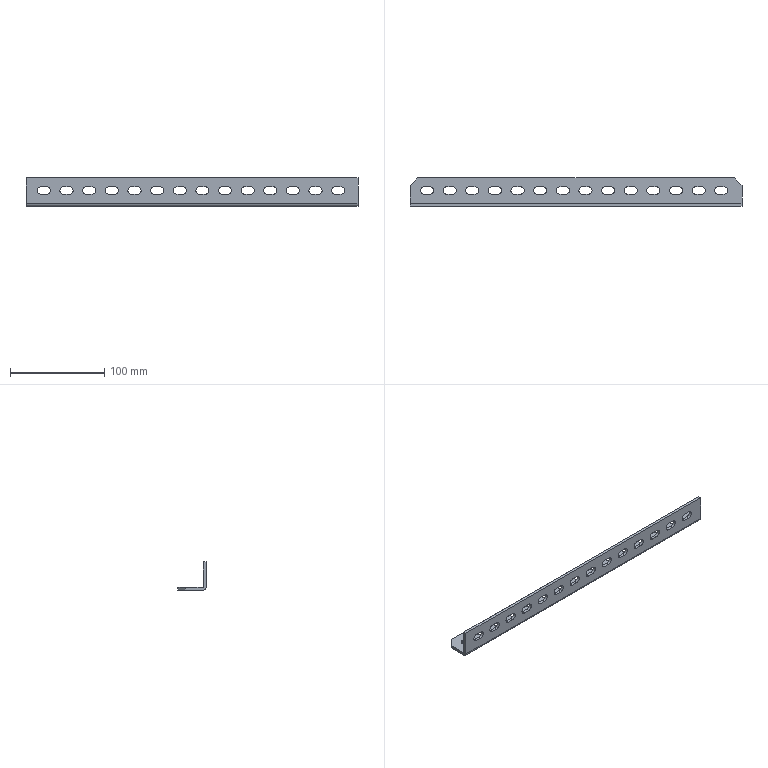Part | SolidWorks | features ICE 3, Cut 1, Extrusion 1, Fillet 1 | 1 solid | 137 faces | box 352 x 30 x 30 mm | volume 51066 mm3 | cylinder 71 | plane 66 | commonest cylinder face diameters 8 x70 6 x1